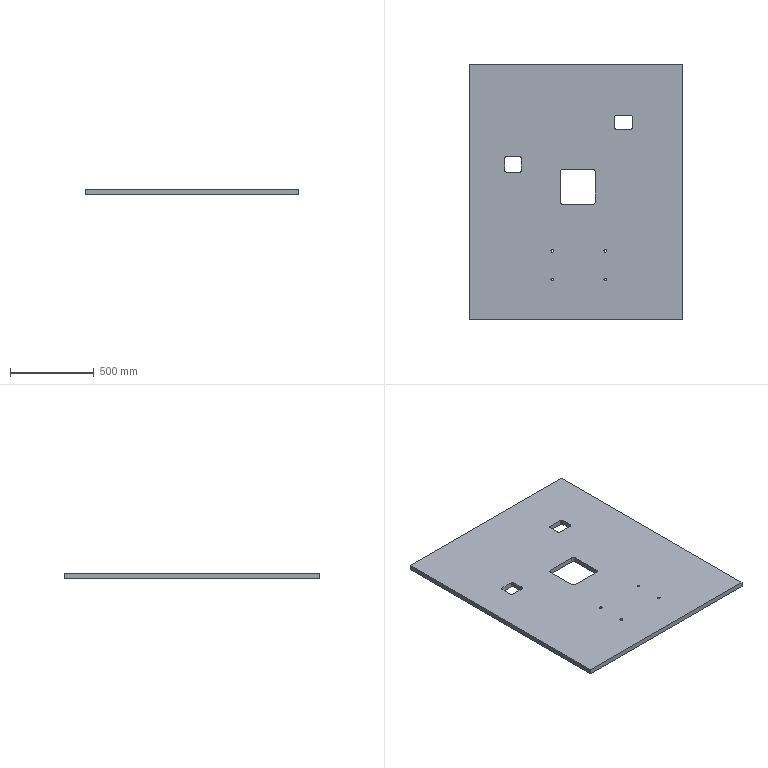Part | STEP file | ASND-0110-Body 1 | 1 solid | 46 faces | box 1280 x 1530 x 30 mm | volume 56875320 mm3 | cylinder 28 | plane 18 | commonest cylinder face diameters 20 x16 16 x8 30 x4